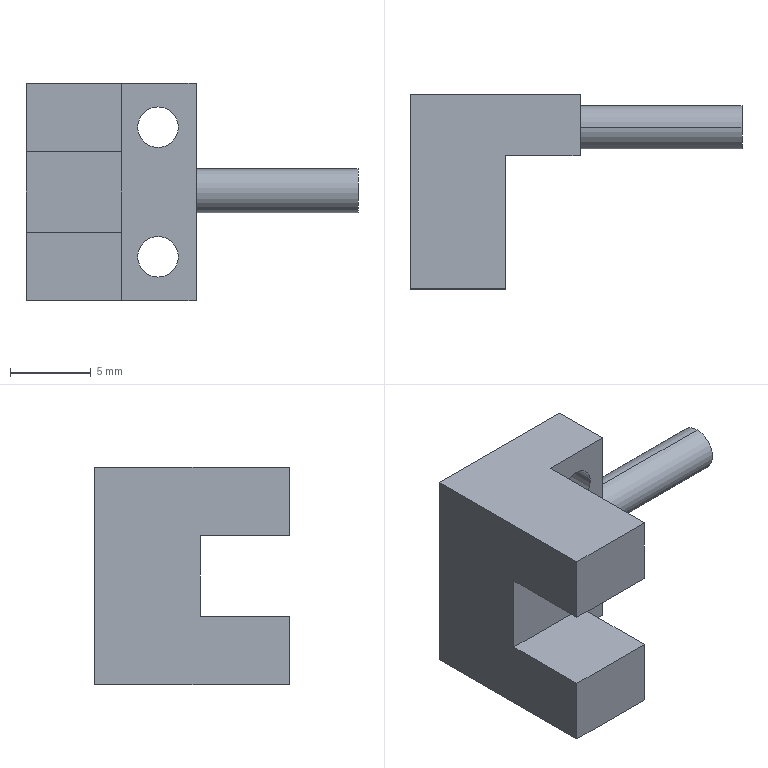Part | STEP file | small slot-type switch DC-SPX205 | 1 solid | 61 faces | box 20.5 x 12 x 13.4 mm | volume 1038 mm3 | plane 42 | spline 13 | cylinder 6 | commonest cylinder face diameters 2.5 x4 2.7 x2